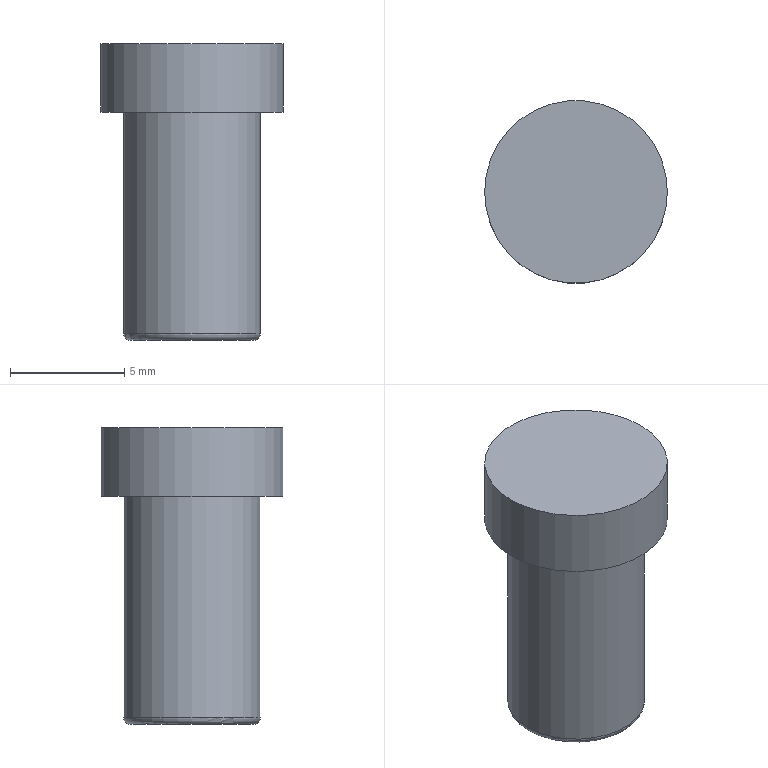Part | STEP file | gslz 2016.10.28-10_id1690_x_t | 1 solid | 6 faces | box 8 x 8 x 13 mm | volume 433.184 mm3 | plane 3 | cylinder 2 | torus 1 | commonest cylinder face diameters 6 x1 8 x1
STEP:
#1=CARTESIAN_POINT('',(0.,0.,0.));
#2=DIRECTION('',(0.,0.,1.));
#3=DIRECTION('',(1.,0.,0.));
#4=AXIS2_PLACEMENT_3D('',#1,#2,#3);
#5=CARTESIAN_POINT('',(871.,40.,10.));
#6=VERTEX_POINT('',#5);
#7=CARTESIAN_POINT('',(879.,40.,10.));
#8=VERTEX_POINT('',#7);
#9=CARTESIAN_POINT('',(875.,40.,10.));
#10=DIRECTION('',(0.,0.,1.));
#11=DIRECTION('',(-1.,0.,0.));
#12=AXIS2_PLACEMENT_3D('',#9,#10,#11);
#13=CIRCLE('',#12,4.);
#14=CARTESIAN_POINT('',(875.,40.,10.));
#15=DIRECTION('',(0.,0.,1.));
#16=DIRECTION('',(-1.,0.,0.));
#17=AXIS2_PLACEMENT_3D('',#14,#15,#16);
#18=PLANE('',#17);
#19=CARTESIAN_POINT('',(0.,0.));
#20=DIRECTION('',(1.,0.));
#21=AXIS2_PLACEMENT_2D('',#19,#20);
#22=CIRCLE('',#21,4.);
#23=(GEOMETRIC_REPRESENTATION_CONTEXT(2)PARAMETRIC_REPRESENTATION_CONTEXT()REPRESENTATION_CONTEXT('',''));
#24=DEFINITIONAL_REPRESENTATION('',(#22),#23);
#25=PCURVE('',#18,#24);
#26=CARTESIAN_POINT('',(875.,40.,10.));
#27=DIRECTION('',(0.,0.,-1.));
#28=DIRECTION('',(1.,0.,0.));
#29=AXIS2_PLACEMENT_3D('',#26,#27,#28);
#30=CYLINDRICAL_SURFACE('',#29,4.);
#31=CARTESIAN_POINT('',(3.142,0.));
#32=DIRECTION('',(-1.,0.));
#33=VECTOR('',#32,1.);
#34=LINE('',#31,#33);
#35=(GEOMETRIC_REPRESENTATION_CONTEXT(2)PARAMETRIC_REPRESENTATION_CONTEXT()REPRESENTATION_CONTEXT('',''));
#36=DEFINITIONAL_REPRESENTATION('',(#34),#35);
#37=PCURVE('',#30,#36);
#38=SURFACE_CURVE('',#13,(#25,#37),.PCURVE_S1.);
#39=EDGE_CURVE('',#6,#8,#38,.T.);
#40=ORIENTED_EDGE('',*,*,#39,.T.);
#41=CARTESIAN_POINT('',(875.,40.,10.));
#42=DIRECTION('',(0.,0.,1.));
#43=DIRECTION('',(-1.,0.,0.));
#44=AXIS2_PLACEMENT_3D('',#41,#42,#43);
#45=CIRCLE('',#44,4.);
#46=CARTESIAN_POINT('',(0.,0.));
#47=DIRECTION('',(1.,0.));
#48=AXIS2_PLACEMENT_2D('',#46,#47);
#49=CIRCLE('',#48,4.);
#50=(GEOMETRIC_REPRESENTATION_CONTEXT(2)PARAMETRIC_REPRESENTATION_CONTEXT()REPRESENTATION_CONTEXT('',''));
#51=DEFINITIONAL_REPRESENTATION('',(#49),#50);
#52=PCURVE('',#18,#51);
#53=CARTESIAN_POINT('',(9.425,0.));
#54=DIRECTION('',(-1.,0.));
#55=VECTOR('',#54,1.);
#56=LINE('',#53,#55);
#57=(GEOMETRIC_REPRESENTATION_CONTEXT(2)PARAMETRIC_REPRESENTATION_CONTEXT()REPRESENTATION_CONTEXT('',''));
#58=DEFINITIONAL_REPRESENTATION('',(#56),#57);
#59=PCURVE('',#30,#58);
#60=SURFACE_CURVE('',#45,(#52,#59),.PCURVE_S1.);
#61=EDGE_CURVE('',#8,#6,#60,.T.);
#62=ORIENTED_EDGE('',*,*,#61,.T.);
#63=EDGE_LOOP('',(#40,#62));
#64=FACE_BOUND('',#63,.T.);
#65=ADVANCED_FACE('',(#64),#18,.T.);
#66=CARTESIAN_POINT('',(878.,40.,7.));
#67=VERTEX_POINT('',#66);
#68=CARTESIAN_POINT('',(875.,40.,7.));
#69=DIRECTION('',(0.,0.,1.));
#70=DIRECTION('',(1.,0.,0.));
#71=AXIS2_PLACEMENT_3D('',#68,#69,#70);
#72=CIRCLE('',#71,3.);
#73=CARTESIAN_POINT('',(875.,40.,7.));
#74=DIRECTION('',(0.,0.,-1.));
#75=DIRECTION('',(1.,0.,0.));
#76=AXIS2_PLACEMENT_3D('',#73,#74,#75);
#77=PLANE('',#76);
#78=CARTESIAN_POINT('',(3.,0.));
#79=CARTESIAN_POINT('',(3.,-5.196));
#80=CARTESIAN_POINT('',(-1.5,-2.598));
#81=CARTESIAN_POINT('',(-6.,0.));
#82=CARTESIAN_POINT('',(-1.5,2.598));
#83=CARTESIAN_POINT('',(3.,5.196));
#84=CARTESIAN_POINT('',(3.,0.));
#85=(BOUNDED_CURVE()B_SPLINE_CURVE(2,(#78,#79,#80,#81,#82,#83,#84),.UNSPECIFIED.,.T.,.F.)B_SPLINE_CURVE_WITH_KNOTS((1,2,2,2,2,1),(-2.094,0.,2.094,4.189,6.283,8.378),.UNSPECIFIED.)CURVE()GEOMETRIC_REPRESENTATION_ITEM()RATIONAL_B_SPLINE_CURVE((1.,0.5,1.,0.5,1.,0.5,1.))REPRESENTATION_ITEM(''));
#86=(GEOMETRIC_REPRESENTATION_CONTEXT(2)PARAMETRIC_REPRESENTATION_CONTEXT()REPRESENTATION_CONTEXT('',''));
#87=DEFINITIONAL_REPRESENTATION('',(#85),#86);
#88=PCURVE('',#77,#87);
#89=CARTESIAN_POINT('',(875.,40.,19.));
#90=DIRECTION('',(0.,0.,-1.));
#91=DIRECTION('',(1.,0.,0.));
#92=AXIS2_PLACEMENT_3D('',#89,#90,#91);
#93=CYLINDRICAL_SURFACE('',#92,3.);
#94=CARTESIAN_POINT('',(6.283,12.));
#95=DIRECTION('',(-1.,0.));
#96=VECTOR('',#95,1.);
#97=LINE('',#94,#96);
#98=(GEOMETRIC_REPRESENTATION_CONTEXT(2)PARAMETRIC_REPRESENTATION_CONTEXT()REPRESENTATION_CONTEXT('',''));
#99=DEFINITIONAL_REPRESENTATION('',(#97),#98);
#100=PCURVE('',#93,#99);
#101=SURFACE_CURVE('',#72,(#88,#100),.PCURVE_S1.);
#102=EDGE_CURVE('',#67,#67,#101,.T.);
#103=ORIENTED_EDGE('',*,*,#102,.T.);
#104=EDGE_LOOP('',(#103));
#105=FACE_BOUND('',#104,.T.);
#106=CARTESIAN_POINT('',(879.,40.,7.));
#107=VERTEX_POINT('',#106);
#108=CARTESIAN_POINT('',(875.,40.,7.));
#109=DIRECTION('',(0.,0.,-1.));
#110=DIRECTION('',(1.,0.,0.));
#111=AXIS2_PLACEMENT_3D('',#108,#109,#110);
#112=CIRCLE('',#111,4.);
#113=CARTESIAN_POINT('',(0.,0.));
#114=DIRECTION('',(1.,0.));
#115=AXIS2_PLACEMENT_2D('',#113,#114);
#116=CIRCLE('',#115,4.);
#117=(GEOMETRIC_REPRESENTATION_CONTEXT(2)PARAMETRIC_REPRESENTATION_CONTEXT()REPRESENTATION_CONTEXT('',''));
#118=DEFINITIONAL_REPRESENTATION('',(#116),#117);
#119=PCURVE('',#77,#118);
#120=CARTESIAN_POINT('',(0.,3.));
#121=DIRECTION('',(1.,0.));
#122=VECTOR('',#121,1.);
#123=LINE('',#120,#122);
#124=(GEOMETRIC_REPRESENTATION_CONTEXT(2)PARAMETRIC_REPRESENTATION_CONTEXT()REPRESENTATION_CONTEXT('',''));
#125=DEFINITIONAL_REPRESENTATION('',(#123),#124);
#126=PCURVE('',#30,#125);
#127=SURFACE_CURVE('',#112,(#119,#126),.PCURVE_S1.);
#128=EDGE_CURVE('',#107,#107,#127,.T.);
#129=ORIENTED_EDGE('',*,*,#128,.T.);
#130=EDGE_LOOP('',(#129));
#131=FACE_BOUND('',#130,.T.);
#132=ADVANCED_FACE('',(#105,#131),#77,.T.);
#133=ORIENTED_EDGE('',*,*,#128,.F.);
#134=CARTESIAN_POINT('',(879.,40.,10.));
#135=CARTESIAN_POINT('',(879.,40.,7.));
#136=B_SPLINE_CURVE_WITH_KNOTS('',1,(#134,#135),.UNSPECIFIED.,.F.,.F.,(2,2),(0.,3.),.PIECEWISE_BEZIER_KNOTS.);
#137=CARTESIAN_POINT('',(0.,0.));
#138=DIRECTION('',(0.,1.));
#139=VECTOR('',#138,1.);
#140=LINE('',#137,#139);
#141=(GEOMETRIC_REPRESENTATION_CONTEXT(2)PARAMETRIC_REPRESENTATION_CONTEXT()REPRESENTATION_CONTEXT('',''));
#142=DEFINITIONAL_REPRESENTATION('',(#140),#141);
#143=PCURVE('',#30,#142);
#144=CARTESIAN_POINT('',(6.283,0.));
#145=DIRECTION('',(0.,1.));
#146=VECTOR('',#145,1.);
#147=LINE('',#144,#146);
#148=(GEOMETRIC_REPRESENTATION_CONTEXT(2)PARAMETRIC_REPRESENTATION_CONTEXT()REPRESENTATION_CONTEXT('',''));
#149=DEFINITIONAL_REPRESENTATION('',(#147),#148);
#150=PCURVE('',#30,#149);
#151=SEAM_CURVE('',#136,(#143,#150),.PCURVE_S1.);
#152=EDGE_CURVE('',#8,#107,#151,.T.);
#153=ORIENTED_EDGE('',*,*,#152,.F.);
#154=ORIENTED_EDGE('',*,*,#39,.F.);
#155=ORIENTED_EDGE('',*,*,#61,.F.);
#156=ORIENTED_EDGE('',*,*,#152,.T.);
#157=EDGE_LOOP('',(#133,#153,#154,#155,#156));
#158=FACE_BOUND('',#157,.T.);
#159=ADVANCED_FACE('',(#158),#30,.T.);
#160=CARTESIAN_POINT('',(872.3,40.,-3.));
#161=VERTEX_POINT('',#160);
#162=CARTESIAN_POINT('',(875.,40.,-3.));
#163=DIRECTION('',(0.,0.,1.));
#164=DIRECTION('',(1.,0.,0.));
#165=AXIS2_PLACEMENT_3D('',#162,#163,#164);
#166=CIRCLE('',#165,2.7);
#167=CARTESIAN_POINT('',(875.,40.,-3.));
#168=DIRECTION('',(0.,0.,-1.));
#169=DIRECTION('',(1.,0.,0.));
#170=AXIS2_PLACEMENT_3D('',#167,#168,#169);
#171=PLANE('',#170);
#172=CARTESIAN_POINT('',(2.7,0.));
#173=CARTESIAN_POINT('',(2.7,-4.677));
#174=CARTESIAN_POINT('',(-1.35,-2.338));
#175=CARTESIAN_POINT('',(-5.4,0.));
#176=CARTESIAN_POINT('',(-1.35,2.338));
#177=CARTESIAN_POINT('',(2.7,4.677));
#178=CARTESIAN_POINT('',(2.7,0.));
#179=(BOUNDED_CURVE()B_SPLINE_CURVE(2,(#172,#173,#174,#175,#176,#177,#178),.UNSPECIFIED.,.T.,.F.)B_SPLINE_CURVE_WITH_KNOTS((1,2,2,2,2,1),(-2.094,0.,2.094,4.189,6.283,8.378),.UNSPECIFIED.)CURVE()GEOMETRIC_REPRESENTATION_ITEM()RATIONAL_B_SPLINE_CURVE((1.,0.5,1.,0.5,1.,0.5,1.))REPRESENTATION_ITEM(''));
#180=(GEOMETRIC_REPRESENTATION_CONTEXT(2)PARAMETRIC_REPRESENTATION_CONTEXT()REPRESENTATION_CONTEXT('',''));
#181=DEFINITIONAL_REPRESENTATION('',(#179),#180);
#182=PCURVE('',#171,#181);
#183=CARTESIAN_POINT('',(875.,40.,-2.7));
#184=DIRECTION('',(0.,0.,-1.));
#185=DIRECTION('',(-1.,0.,0.));
#186=AXIS2_PLACEMENT_3D('',#183,#184,#185);
#187=TOROIDAL_SURFACE('',#186,2.7,0.3);
#188=CARTESIAN_POINT('',(9.425,7.854));
#189=DIRECTION('',(-1.,0.));
#190=VECTOR('',#189,1.);
#191=LINE('',#188,#190);
#192=(GEOMETRIC_REPRESENTATION_CONTEXT(2)PARAMETRIC_REPRESENTATION_CONTEXT()REPRESENTATION_CONTEXT('',''));
#193=DEFINITIONAL_REPRESENTATION('',(#191),#192);
#194=PCURVE('',#187,#193);
#195=SURFACE_CURVE('',#166,(#182,#194),.PCURVE_S1.);
#196=EDGE_CURVE('',#161,#161,#195,.T.);
#197=ORIENTED_EDGE('',*,*,#196,.F.);
#198=EDGE_LOOP('',(#197));
#199=FACE_BOUND('',#198,.T.);
#200=ADVANCED_FACE('',(#199),#171,.T.);
#201=CARTESIAN_POINT('',(878.,40.,-2.7));
#202=VERTEX_POINT('',#201);
#203=CARTESIAN_POINT('',(872.,40.,-2.7));
#204=VERTEX_POINT('',#203);
#205=CARTESIAN_POINT('',(875.,40.,-2.7));
#206=DIRECTION('',(0.,0.,-1.));
#207=DIRECTION('',(1.,0.,0.));
#208=AXIS2_PLACEMENT_3D('',#205,#206,#207);
#209=CIRCLE('',#208,3.);
#210=CARTESIAN_POINT('',(0.,21.7));
#211=DIRECTION('',(1.,0.));
#212=VECTOR('',#211,1.);
#213=LINE('',#210,#212);
#214=(GEOMETRIC_REPRESENTATION_CONTEXT(2)PARAMETRIC_REPRESENTATION_CONTEXT()REPRESENTATION_CONTEXT('',''));
#215=DEFINITIONAL_REPRESENTATION('',(#213),#214);
#216=PCURVE('',#93,#215);
#217=CARTESIAN_POINT('',(3.142,6.283));
#218=DIRECTION('',(1.,0.));
#219=VECTOR('',#218,1.);
#220=LINE('',#217,#219);
#221=(GEOMETRIC_REPRESENTATION_CONTEXT(2)PARAMETRIC_REPRESENTATION_CONTEXT()REPRESENTATION_CONTEXT('',''));
#222=DEFINITIONAL_REPRESENTATION('',(#220),#221);
#223=PCURVE('',#187,#222);
#224=SURFACE_CURVE('',#209,(#216,#223),.PCURVE_S1.);
#225=EDGE_CURVE('',#202,#204,#224,.T.);
#226=ORIENTED_EDGE('',*,*,#225,.F.);
#227=CARTESIAN_POINT('',(878.,40.,7.));
#228=CARTESIAN_POINT('',(878.,40.,-2.7));
#229=B_SPLINE_CURVE_WITH_KNOTS('',1,(#227,#228),.UNSPECIFIED.,.F.,.F.,(2,2),(12.,21.7),.PIECEWISE_BEZIER_KNOTS.);
#230=CARTESIAN_POINT('',(0.,0.));
#231=DIRECTION('',(0.,1.));
#232=VECTOR('',#231,1.);
#233=LINE('',#230,#232);
#234=(GEOMETRIC_REPRESENTATION_CONTEXT(2)PARAMETRIC_REPRESENTATION_CONTEXT()REPRESENTATION_CONTEXT('',''));
#235=DEFINITIONAL_REPRESENTATION('',(#233),#234);
#236=PCURVE('',#93,#235);
#237=CARTESIAN_POINT('',(6.283,0.));
#238=DIRECTION('',(0.,1.));
#239=VECTOR('',#238,1.);
#240=LINE('',#237,#239);
#241=(GEOMETRIC_REPRESENTATION_CONTEXT(2)PARAMETRIC_REPRESENTATION_CONTEXT()REPRESENTATION_CONTEXT('',''));
#242=DEFINITIONAL_REPRESENTATION('',(#240),#241);
#243=PCURVE('',#93,#242);
#244=SEAM_CURVE('',#229,(#236,#243),.PCURVE_S1.);
#245=EDGE_CURVE('',#67,#202,#244,.T.);
#246=ORIENTED_EDGE('',*,*,#245,.F.);
#247=ORIENTED_EDGE('',*,*,#102,.F.);
#248=ORIENTED_EDGE('',*,*,#245,.T.);
#249=CARTESIAN_POINT('',(875.,40.,-2.7));
#250=DIRECTION('',(0.,0.,-1.));
#251=DIRECTION('',(1.,0.,0.));
#252=AXIS2_PLACEMENT_3D('',#249,#250,#251);
#253=CIRCLE('',#252,3.);
#254=CARTESIAN_POINT('',(0.,21.7));
#255=DIRECTION('',(1.,0.));
#256=VECTOR('',#255,1.);
#257=LINE('',#254,#256);
#258=(GEOMETRIC_REPRESENTATION_CONTEXT(2)PARAMETRIC_REPRESENTATION_CONTEXT()REPRESENTATION_CONTEXT('',''));
#259=DEFINITIONAL_REPRESENTATION('',(#257),#258);
#260=PCURVE('',#93,#259);
#261=CARTESIAN_POINT('',(-3.142,6.283));
#262=DIRECTION('',(1.,0.));
#263=VECTOR('',#262,1.);
#264=LINE('',#261,#263);
#265=(GEOMETRIC_REPRESENTATION_CONTEXT(2)PARAMETRIC_REPRESENTATION_CONTEXT()REPRESENTATION_CONTEXT('',''));
#266=DEFINITIONAL_REPRESENTATION('',(#264),#265);
#267=PCURVE('',#187,#266);
#268=SURFACE_CURVE('',#253,(#260,#267),.PCURVE_S1.);
#269=EDGE_CURVE('',#204,#202,#268,.T.);
#270=ORIENTED_EDGE('',*,*,#269,.F.);
#271=EDGE_LOOP('',(#226,#246,#247,#248,#270));
#272=FACE_BOUND('',#271,.T.);
#273=ADVANCED_FACE('',(#272),#93,.T.);
#274=ORIENTED_EDGE('',*,*,#196,.T.);
#275=CARTESIAN_POINT('',(872.,40.,-2.7));
#276=CARTESIAN_POINT('',(872.,40.,-2.78));
#277=CARTESIAN_POINT('',(872.026,40.,-2.858));
#278=CARTESIAN_POINT('',(872.074,40.,-2.926));
#279=CARTESIAN_POINT('',(872.142,40.,-2.974));
#280=CARTESIAN_POINT('',(872.22,40.,-3.));
#281=CARTESIAN_POINT('',(872.3,40.,-3.));
#282=(BOUNDED_CURVE()B_SPLINE_CURVE(6,(#275,#276,#277,#278,#279,#280,#281),.UNSPECIFIED.,.F.,.F.)B_SPLINE_CURVE_WITH_KNOTS((7,7),(0.,1.571),.PIECEWISE_BEZIER_KNOTS.)CURVE()GEOMETRIC_REPRESENTATION_ITEM()RATIONAL_B_SPLINE_CURVE((1.031,1.01,0.9979,0.994,0.9979,1.01,1.031))REPRESENTATION_ITEM(''));
#283=CARTESIAN_POINT('',(0.,6.283));
#284=DIRECTION('',(0.,1.));
#285=VECTOR('',#284,1.);
#286=LINE('',#283,#285);
#287=(GEOMETRIC_REPRESENTATION_CONTEXT(2)PARAMETRIC_REPRESENTATION_CONTEXT()REPRESENTATION_CONTEXT('',''));
#288=DEFINITIONAL_REPRESENTATION('',(#286),#287);
#289=PCURVE('',#187,#288);
#290=CARTESIAN_POINT('',(6.283,6.283));
#291=DIRECTION('',(0.,1.));
#292=VECTOR('',#291,1.);
#293=LINE('',#290,#292);
#294=(GEOMETRIC_REPRESENTATION_CONTEXT(2)PARAMETRIC_REPRESENTATION_CONTEXT()REPRESENTATION_CONTEXT('',''));
#295=DEFINITIONAL_REPRESENTATION('',(#293),#294);
#296=PCURVE('',#187,#295);
#297=SEAM_CURVE('',#282,(#289,#296),.PCURVE_S1.);
#298=EDGE_CURVE('',#204,#161,#297,.T.);
#299=ORIENTED_EDGE('',*,*,#298,.F.);
#300=ORIENTED_EDGE('',*,*,#269,.T.);
#301=ORIENTED_EDGE('',*,*,#225,.T.);
#302=ORIENTED_EDGE('',*,*,#298,.T.);
#303=EDGE_LOOP('',(#274,#299,#300,#301,#302));
#304=FACE_BOUND('',#303,.T.);
#305=ADVANCED_FACE('',(#304),#187,.T.);
#306=CLOSED_SHELL('',(#65,#132,#159,#200,#273,#305));
#307=MANIFOLD_SOLID_BREP('',#306);
#308=(LENGTH_UNIT()NAMED_UNIT(*)SI_UNIT(.MILLI.,.METRE.));
#309=UNCERTAINTY_MEASURE_WITH_UNIT(LENGTH_MEASURE(0.000005),#308,'','');
#310=(NAMED_UNIT(*)PLANE_ANGLE_UNIT()SI_UNIT($,.RADIAN.));
#311=(NAMED_UNIT(*)SI_UNIT($,.STERADIAN.)SOLID_ANGLE_UNIT());
#312=(GEOMETRIC_REPRESENTATION_CONTEXT(3)GLOBAL_UNCERTAINTY_ASSIGNED_CONTEXT((#309))GLOBAL_UNIT_ASSIGNED_CONTEXT((#308,#310,#311))REPRESENTATION_CONTEXT('',''));
#313=ADVANCED_BREP_SHAPE_REPRESENTATION('',(#4,#307),#312);